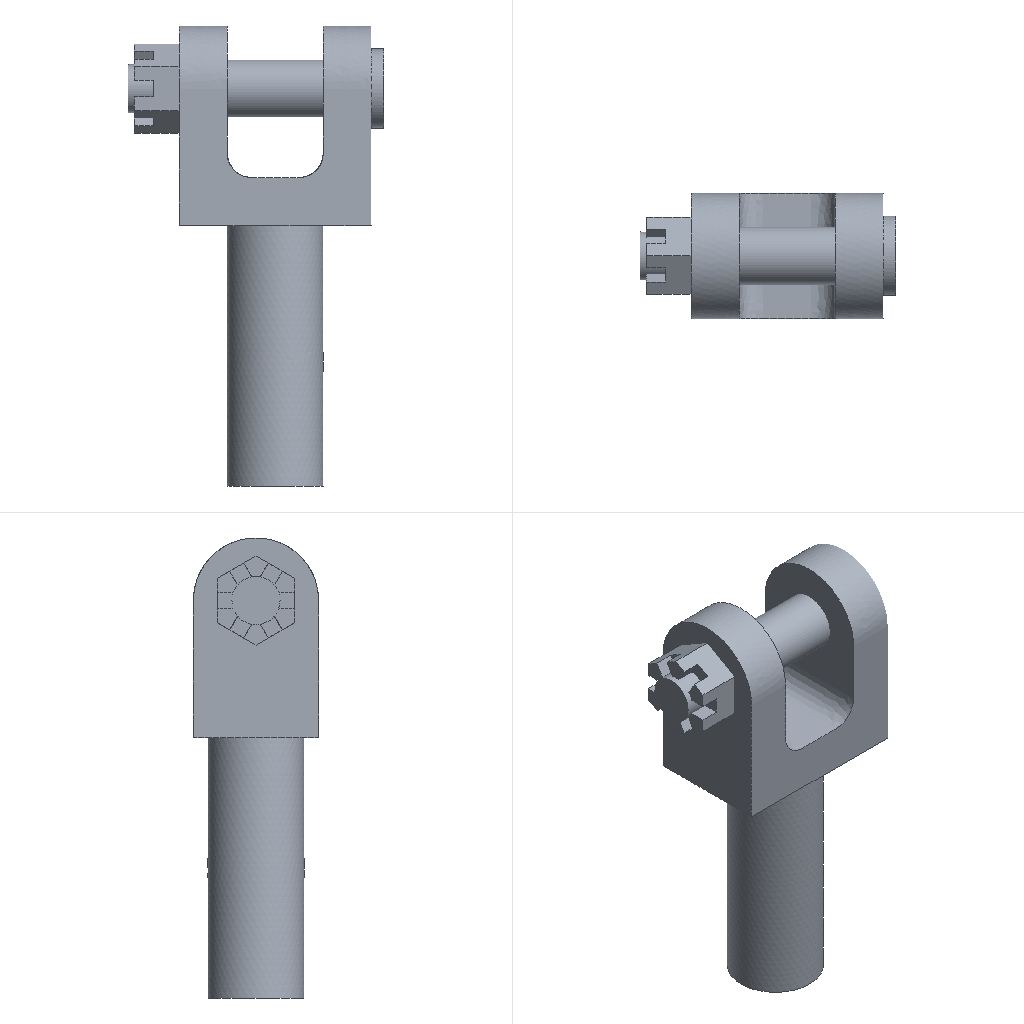Simulation study | ansys workbench
Set-up summary:
category,name,step,type,value,unit,region
solver,ansys_workbench
units,mm-N-s-tonne (MPa),,stated,"/units,MPA"
analysis,LS1,,static
load_step,LS1,LS1,static,nsubst=1; time=1
mesh,nodes,,,248082
mesh,elements,,,141187
element_type,SOLID187,,,108372
element_type,SOLID186,,,20185
element_type,TARGE170,,,5715
element_type,CONTA174,,,5715
element_type,SURF154,,,1200
material,Special steel,,E,200000,tonne s^-2 mm^-1
material,Special steel,,nu,0.3
material,Special steel,,density,7.85e-09,tonne mm^-3
load,Create Bearing Load,LS1,surface-effect pres face 5,65500,,SURF154 #12
bc,Fixed Supports,model,fixed,[dofs=ALL],,_FIXEDSU
bc,"Construct Weak Springs, Prototype 1",model,fixed,[dofs=ALL n=3],,node list
bc,"Construct Weak Springs, Prototype 2",model,fixed,[dofs=ALL n=3],,node list
bc,"Construct Weak Springs, Prototype 3",model,fixed,[dofs=ALL n=3],,node list
contact,Bonded - part.1 To part.2,,bonded (always),element=CONTA174
contact,Bonded - part.1 To part.3,,bonded (always),element=CONTA174
contact,Frictionless - part.3 To part.1,,standard (frictionless/frictional),element=CONTA174
contact,Bonded - part.3 To part.2,,bonded (always),element=CONTA174
named_set,_FIXEDSU,,node,6972
Ansys APDL input file, long lists of numbers shortened:
/batch
/config,noeldb,1     ! force off writing results to database
*get,_wallstrt,active,,time,wall
! ANSYS input file written by Workbench version 17.0 RELEASE
! File used for geometry attach:
/title,Hinge_pin_analysis--Static Structural (A5)
*DIM,_wb_ProjectScratch_dir,string,248
_wb_ProjectScratch_dir(1) = ''
*DIM,_wb_SolverFiles_dir,string,248
_wb_SolverFiles_dir(1) = ''
*DIM,_wb_userfiles_dir,string,248
_wb_userfiles_dir(1) = ''
/com,--- Data in consistent NMM units. See Solving Units in the help system for more information.
/units,MPA
/nopr
/wb,file,start              !  signify a WB generated input file
/prep7
! Turn off shape checking because checks already performed inside WB mesher.
! See help system for more information.
SHPP,OFF,,NOWARN
/nolist
etcon,set             ! allow ANSYS to choose best KEYOP's for 180x elements
/com,*********** Nodes for the whole assembly ***********
nblock,3
(1i9,3e20.9e3)
    88057   -2.930000000E+001   -2.527756814E+000    7.482179677E+001
! (248081 more lines like these left out)
-1
/wb,elem,start            !  set before creation of elements
/com,*********** Elements for Body 1 "part.1" ***********
et,1,187
eblock,19,solid,,98306
(19i9)
        1        1        1        1        0        0        0        0       10        0    30252   108013   108036   110488   110487   150708   150871   150712   150711
! (196611 more lines like these left out)
-1
/com,*********** Elements for Body 2 "part.2" ***********
et,2,187
eblock,19,solid,,10066
(19i9)
        2        2        2        2        0        0        0        0       10        0    20186    89367    90267    89959    90136    98772   102626    98769    98771
! (20131 more lines like these left out)
-1
/com,*********** Elements for Body 3 "part.3" ***********
et,3,186
keyo,3,2,1          ! set full integration on SOLID186
eblock,19,solid,,20185
(19i9)
        3        3        3        3        0        0        0        0       20        0   128558   270364   270368   270458   270457   270640   270644   270734   270733
! (40369 more lines like these left out)
-1
/wb,elem,end               !  done creating elements
/com,*********** Send User Defined Coordinate System(s) ***********
csys,0
toffst,273.15,  ! Temperature offset from absolute zero
/com,*********** Set Reference Temperature ***********
tref,22.
/wb,mat,start              !  starting to send materials
/com,*********** Send Materials ***********
MP,DENS,1,7.85e-09,	! tonne mm^-3
MP,EX,1,200000,	! tonne s^-2 mm^-1
MP,NUXY,1,0.3,
MP,DENS,2,7.85e-09,	! tonne mm^-3
MP,EX,2,200000,	! tonne s^-2 mm^-1
MP,NUXY,2,0.3,
MP,DENS,3,7.85e-09,	! tonne mm^-3
MP,EX,3,200000,	! tonne s^-2 mm^-1
MP,NUXY,3,0.3,
/wb,mat,end                !  done sending materials
!************************* Model Summary ********************
!part.1,	Special steel,	matid,	1
!part.2,	Special steel,	matid,	2
!part.3,	Special steel,	matid,	3
!************************* End Model Summary ********************
! get the diagonal of the bounding box. Needed later for other things
*get,_xmin,node,,mnloc,x
*get,_ymin,node,,mnloc,y
*get,_zmin,node,,mnloc,z
*get,_xmax,node,,mxloc,x
*get,_ymax,node,,mxloc,y
*get,_zmax,node,,mxloc,z
_ASMDIAG=(_xmax-_xmin)*(_xmax-_xmin)+(_ymax-_ymin)*(_ymax-_ymin)+(_zmax-_zmin)*(_zmax-_zmin)
_ASMDIAG=SQRT(_ASMDIAG)
/wb,contact,start          !  starting to send contact
/com,*********** Create Contact "Bonded - part.1 To part.2" ***********
/com,            Real Constant Set For Above Contact Is 5 & 4
*set,tid,5
*set,cid,4
r,tid
r,cid
et,tid,170
et,cid,174
eblock,10,,,201
(15i9)
   148743        5        5        5        0   109561   109894   109667   109667   161297   162289   109667   161294
! (200 more lines like these left out)
-1
eblock,10,,,201
(15i9)
   148944        4        4        4        0   109561   109894   109667   109667   161297   162289   109667   161294
! (200 more lines like these left out)
-1
eblock,10,,,318
(15i9)
   149145        4        5        4        0    88662    88692    88681    88681    94560    94724    88681    94558
! (317 more lines like these left out)
-1
eblock,10,,,318
(15i9)
   149463        5        4        5        0    88662    88692    88681    88681    94560    94724    88681    94558
! (317 more lines like these left out)
-1
keyo,cid,8,2               ! auto create asymmetric contact (from Program Controlled setting)
keyo,cid,10,2              ! adjust contact stiffness each NR iteration (from Program Controlled setting)
keyo,cid,12,5              ! bonded always
keyo,cid,2,0               ! augmented Lagrange (from Program Controlled setting)
keyo,cid,4,0               ! on Gauss point (from Program Controlled setting)
keyo,cid,9,1               ! ignore initial gaps/penetration
keyo,cid,7,0               ! No Prediction
rmod,tid,3,1.	! FKN
rmod,tid,5,0.	! ICONT
rmod,tid,6,0.	! PINB
rmod,tid,10,0.	! CNOF
rmod,tid,12,0.	! FKT
rmod,tid,36,455	! WB DSID
rmod,cid,3,1.	! FKN
rmod,cid,5,0.	! ICONT
rmod,cid,6,0.	! PINB
rmod,cid,10,0.	! CNOF
rmod,cid,12,0.	! FKT
rmod,cid,36,455	! WB DSID
/com,*********** Create Contact "Bonded - part.1 To part.3" ***********
/com,            Real Constant Set For Above Contact Is 7 & 6
*set,tid,7
*set,cid,6
r,tid
r,cid
et,tid,170
et,cid,174
eblock,10,,,870
(15i9)
   149781        7        7        7        0   108776   109073   108950   108950   156013   157507   108950   156011
! (869 more lines like these left out)
-1
eblock,10,,,870
(15i9)
   150651        6        6        6        0   108776   109073   108950   108950   156013   157507   108950   156011
! (869 more lines like these left out)
-1
eblock,10,,,120
(15i9)
   151521        6        7        6        0   248190   248189   248434   248441   271549   272020   272040   270858
! (119 more lines like these left out)
-1
eblock,10,,,120
(15i9)
   151641        7        6        7        0   248190   248189   248434   248441   271549   272020   272040   270858
! (119 more lines like these left out)
-1
keyo,cid,8,2               ! auto create asymmetric contact (from Program Controlled setting)
keyo,cid,10,2              ! adjust contact stiffness each NR iteration (from Program Controlled setting)
keyo,cid,12,5              ! bonded always
keyo,cid,2,0               ! augmented Lagrange (from Program Controlled setting)
keyo,cid,4,0               ! on Gauss point (from Program Controlled setting)
keyo,cid,9,1               ! ignore initial gaps/penetration
keyo,cid,7,0               ! No Prediction
rmod,tid,3,1.	! FKN
rmod,tid,5,0.	! ICONT
rmod,tid,6,0.	! PINB
rmod,tid,10,0.	! CNOF
rmod,tid,12,0.	! FKT
rmod,tid,36,461	! WB DSID
rmod,cid,3,1.	! FKN
rmod,cid,5,0.	! ICONT
rmod,cid,6,0.	! PINB
rmod,cid,10,0.	! CNOF
rmod,cid,12,0.	! FKT
rmod,cid,36,461	! WB DSID
/com,*********** Create Contact "Frictionless - part.3 To part.1" ***********
/com,            Real Constant Set For Above Contact Is 9 & 8
*set,tid,9
*set,cid,8
r,tid
r,cid
et,tid,170
et,cid,174
eblock,10,,,2400
(15i9)
   151761        9        9        9        0   255215   255551   255550   255214   291870   291869   291868   270949
! (2399 more lines like these left out)
-1
eblock,10,,,2400
(15i9)
   154161        8        8        8        0   255215   255551   255550   255214   291870   291869   291868   270949
! (2399 more lines like these left out)
-1
eblock,10,,,728
(15i9)
   156561        8        9        8        0   104315   104417   104210   104210   124699   123907   104210   123906
! (727 more lines like these left out)
-1
eblock,10,,,728
(15i9)
   157289        9        8        9        0   104315   104417   104210   104210   124699   123907   104210   123906
! (727 more lines like these left out)
-1
keyo,cid,8,2               ! auto create asymmetric contact (from Program Controlled setting)
keyo,cid,10,2              ! adjust contact stiffness each NR iteration (from Program Controlled setting)
keyo,cid,12,0              ! standard contact
keyo,cid,2,0               ! augmented Lagrange (from Program Controlled setting)
keyo,cid,4,0               ! on Gauss point (from Program Controlled setting)
keyo,cid,9,0               ! use real geometry with stepped effects
keyo,cid,7,0               ! No Prediction
rmod,tid,3,1.	! FKN
rmod,tid,5,0.	! ICONT
rmod,tid,6,0.	! PINB
rmod,tid,10,0.	! CNOF
rmod,tid,12,0.	! FKT
rmod,tid,36,506	! WB DSID
rmod,cid,3,1.	! FKN
rmod,cid,5,0.	! ICONT
rmod,cid,6,0.	! PINB
rmod,cid,10,0.	! CNOF
rmod,cid,12,0.	! FKT
rmod,cid,36,506	! WB DSID
/com,*********** Create Contact "Bonded - part.3 To part.2" ***********
/com,            Real Constant Set For Above Contact Is 11 & 10
*set,tid,11
*set,cid,10
r,tid
r,cid
et,tid,170
et,cid,174
eblock,10,,,600
(15i9)
   158017       11       11       11        0   248812   248814   248813   248811   272958   272956   272955   271382
! (599 more lines like these left out)
-1
eblock,10,,,600
(15i9)
   158617       10       10       10        0   248812   248814   248813   248811   272958   272956   272955   271382
! (599 more lines like these left out)
-1
eblock,10,,,478
(15i9)
   159217       10       11       10        0    88211    88212    88467    88467    91383    91393    88467    91386
! (477 more lines like these left out)
-1
eblock,10,,,478
(15i9)
   159695       11       10       11        0    88211    88212    88467    88467    91383    91393    88467    91386
! (477 more lines like these left out)
-1
keyo,cid,8,2               ! auto create asymmetric contact (from Program Controlled setting)
keyo,cid,10,2              ! adjust contact stiffness each NR iteration (from Program Controlled setting)
keyo,cid,12,5              ! bonded always
keyo,cid,2,0               ! augmented Lagrange (from Program Controlled setting)
keyo,cid,4,0               ! on Gauss point (from Program Controlled setting)
keyo,cid,9,1               ! ignore initial gaps/penetration
keyo,cid,7,0               ! No Prediction
rmod,tid,3,1.	! FKN
rmod,tid,5,0.	! ICONT
rmod,tid,6,0.	! PINB
rmod,tid,10,0.	! CNOF
rmod,tid,12,0.	! FKT
rmod,tid,36,510	! WB DSID
rmod,cid,3,1.	! FKN
rmod,cid,5,0.	! ICONT
rmod,cid,6,0.	! PINB
rmod,cid,10,0.	! CNOF
rmod,cid,12,0.	! FKT
rmod,cid,36,510	! WB DSID
nsel,all
esel,all
/wb,contact,end            !  done creating contacts
/golist
/wb,load,start             !  starting to send loads
/com,*********** Fixed Supports ***********
CMBLOCK,_FIXEDSU,NODE,     6972
(8i10)
    104728    104729    104730    104731    104732    104733    104734    104735
! (871 more lines like these left out)
cmsel,s,_FIXEDSU
d,all,all
nsel,all
nsel,all
/com,*********** Create Bearing Load ***********
et,12,154
eblock,10,,,1200
(15i9)
   160173       12       12       12        0   255192   255528   255527   255191   291818   291817   270989   271247
! (1199 more lines like these left out)
-1
esel,s,type,,12
keyop,12,7,1                ! Use original area so load is constant in large deformation
esel,all
et,13,14             ! spring element type
/com,*********** Construct Weak Springs, Prototype 1 ***********
*set,_delta,5.342
type,13
mat,14
real,14
r,14,1.45131937772807e-004
nsel,all
*get,_nspr,ndmx
_nspr=_nspr+1
esel,s,mat,,1
nsle,s,active
*get,_minx,node,0,mnloc,x
*get,_miny,node,0,mnloc,y
*get,_minz,node,0,mnloc,z
*get,_maxx,node,0,mxloc,x
*get,_maxy,node,0,mxloc,y
*get,_maxz,node,0,mxloc,z
*dim,_ntets,arra,8
_ntets(1) = NODE(_minx,_miny,_minz)
_ntets(2) = NODE(_minx,_miny,_maxz)
_ntets(3) = NODE(_minx,_maxy,_minz)
_ntets(4) = NODE(_minx,_maxy,_maxz)
_ntets(5) = NODE(_maxx,_miny,_minz)
_ntets(6) = NODE(_maxx,_miny,_maxz)
_ntets(7) = NODE(_maxx,_maxy,_minz)
_ntets(8) = NODE(_maxx,_maxy,_maxz)
*do,_i,1,8
  n,_nspr,nx(_ntets(_i))+_delta,ny(_ntets(_i)),nz(_ntets(_i))
  e,_ntets(_i),_nspr
  d,_nspr,all
  _nspr=_nspr+1
  n,_nspr,nx(_ntets(_i)),ny(_ntets(_i))+_delta,nz(_ntets(_i))
  e,_ntets(_i),_nspr
  d,_nspr,all
  _nspr=_nspr+1
  n,_nspr,nx(_ntets(_i)),ny(_ntets(_i)),nz(_ntets(_i))+_delta
  e,_ntets(_i),_nspr
  d,_nspr,all
  _nspr=_nspr+1
*enddo
*set,_ntets
nsel,all
esel,all
/com,*********** Construct Weak Springs, Prototype 2 ***********
*set,_delta,1.308
type,13
mat,15
real,15
r,15,9.49946830519664e-005
nsel,all
*get,_nspr,ndmx
_nspr=_nspr+1
esel,s,mat,,2
nsle,s,active
*get,_minx,node,0,mnloc,x
*get,_miny,node,0,mnloc,y
*get,_minz,node,0,mnloc,z
*get,_maxx,node,0,mxloc,x
*get,_maxy,node,0,mxloc,y
*get,_maxz,node,0,mxloc,z
*dim,_ntets,arra,8
_ntets(1) = NODE(_minx,_miny,_minz)
_ntets(2) = NODE(_minx,_miny,_maxz)
_ntets(3) = NODE(_minx,_maxy,_minz)
_ntets(4) = NODE(_minx,_maxy,_maxz)
_ntets(5) = NODE(_maxx,_miny,_minz)
_ntets(6) = NODE(_maxx,_miny,_maxz)
_ntets(7) = NODE(_maxx,_maxy,_minz)
_ntets(8) = NODE(_maxx,_maxy,_maxz)
*do,_i,1,8
  n,_nspr,nx(_ntets(_i))+_delta,ny(_ntets(_i)),nz(_ntets(_i))
  e,_ntets(_i),_nspr
  d,_nspr,all
  _nspr=_nspr+1
  n,_nspr,nx(_ntets(_i)),ny(_ntets(_i))+_delta,nz(_ntets(_i))
  e,_ntets(_i),_nspr
  d,_nspr,all
  _nspr=_nspr+1
  n,_nspr,nx(_ntets(_i)),ny(_ntets(_i)),nz(_ntets(_i))+_delta
  e,_ntets(_i),_nspr
  d,_nspr,all
  _nspr=_nspr+1
*enddo
*set,_ntets
nsel,all
esel,all
/com,*********** Construct Weak Springs, Prototype 3 ***********
*set,_delta,2.895
type,13
mat,16
real,16
r,16,1.31071703429123e-004
nsel,all
*get,_nspr,ndmx
_nspr=_nspr+1
esel,s,mat,,3
nsle,s,active
*get,_minx,node,0,mnloc,x
*get,_miny,node,0,mnloc,y
*get,_minz,node,0,mnloc,z
*get,_maxx,node,0,mxloc,x
*get,_maxy,node,0,mxloc,y
*get,_maxz,node,0,mxloc,z
*dim,_ntets,arra,8
_ntets(1) = NODE(_minx,_miny,_minz)
_ntets(2) = NODE(_minx,_miny,_maxz)
_ntets(3) = NODE(_minx,_maxy,_minz)
_ntets(4) = NODE(_minx,_maxy,_maxz)
_ntets(5) = NODE(_maxx,_miny,_minz)
_ntets(6) = NODE(_maxx,_miny,_maxz)
_ntets(7) = NODE(_maxx,_maxy,_minz)
_ntets(8) = NODE(_maxx,_maxy,_maxz)
*do,_i,1,8
  n,_nspr,nx(_ntets(_i))+_delta,ny(_ntets(_i)),nz(_ntets(_i))
  e,_ntets(_i),_nspr
  d,_nspr,all
  _nspr=_nspr+1
  n,_nspr,nx(_ntets(_i)),ny(_ntets(_i))+_delta,nz(_ntets(_i))
  e,_ntets(_i),_nspr
  d,_nspr,all
  _nspr=_nspr+1
  n,_nspr,nx(_ntets(_i)),ny(_ntets(_i)),nz(_ntets(_i))+_delta
  e,_ntets(_i),_nspr
  d,_nspr,all
  _nspr=_nspr+1
*enddo
*set,_ntets
nsel,all
esel,all
/gst,on,on
fini
*get,_numnode,node,0,count
*get,_numelem,elem,0,count
*get, _MAXELEMNUM, elem, 0, NUM, MAX
*get, _MAXNODENUM, node, 0, NUM, MAX
*get, _MAXELEMTYPE, etyp, 0, NUM, MAX
*get, _MAXREALCONST, real, 0, NUM, MAX
/go
/wb,load,end               !  done creating loads
/com,--- Number of total nodes = %_numnode%
/com,--- Number of contact elements = 12630
/com,--- Number of spring elements = 72
/com,--- Number of bearing elements = 0
/com,--- Number of solid elements = 128557
/com,--- Number of total elements = %_numelem%
*get,_wallbsol,active,,time,wall
/com,****************************************************************************
/com,*************************    SOLUTION       ********************************
/com,****************************************************************************
/solu
antype,0                   ! static analysis
eqsl,pcg,1e-8,,,,,,1
cntr,print,1               ! print out contact info and also make no initial contact an error
dmpopt,emat,no             ! Don't combine emat file for DANSYS
dmpopt,esav,no             ! Don't combine esav file for DANSYS
nldiag,cont,iter           ! print out contact info each equilibrium iteration
resc,define,last,last,,dele	   ! Program Controlled
/com,****************************************************
/com,******************* SOLVE FOR LS 1 ****************
esel,s,type,,12
sfe,all,5,pres,0,0.0,1.,0.,0.
local,11,0,0,0,0,90.,0.,-90.
csys,0
*set,_v1,0.
*set,_v2,0.
*set,_v3,1.
*get,_necurr,elem,,count
_ecurr=0
_total=0
*do,_i,1,_necurr
  _ecurr = ELNEXT(_ecurr)
  _normx = NORMNX(NELEM(_ecurr,1),NELEM(_ecurr,2),NELEM(_ecurr,3))
! (7 more lines like these left out)
  *if,_dot,gt,-0.00001,then
    esel,u,elem,,_ecurr
  *else
    csys,11
    *get,_indd,elem,_ecurr,aproj,x
    csys,0
    _total=_total+_indd
  *endif
*enddo
*get,_necurr,elem,,count
*if,_necurr,eq,0,then
  *msg,error
  NO ELEMENTS ARE SELECTED TO APPLY BEARING LOAD TO. &
  IT IS LIKELY THAT THE BEARING LOAD IS IN THE WRONG DIRECTION
*endif
*set,_mag,65500.
_mag=_mag/_total
sfe,all,5,pres,0,_mag,0.,0.,65500.
nsel,all
esel,all
/nopr
/gopr
autots,on                  ! Workbench Program Controlled automatic time stepping
nsub,1,10,1                ! due to presence of general nonlinear
time,1.
outres,erase
outres,all,none
outres,nsol,all
outres,rsol,all
outres,strs,all
outres,epel,all
outres,eppl,all
stabilize,off                   ! Stabilization turned OFF by user
! *********** WB SOLVE COMMAND ***********
! check interactive state
*get,ANSINTER_,active,,int
*if,ANSINTER_,ne,0,then
/eof
*endif
solve
/com *************** Write FE CONNECTORS *********
CEWRITE,file,ce,,INTE
/com,****************************************************
/com,*************** FINISHED SOLVE FOR LS 1 *************
*set,_DS_PROGRESS          ! turn off progress updates to avoid virus scanning bug
*get,_wallasol,active,,time,wall
/nopr
*get,_numnode,node,0,count
*get,_numelem,elem,0,count
*get, _MAXELEMNUM, elem, 0, NUM, MAX
*get, _MAXNODENUM, node, 0, NUM, MAX,,,INTERNAL
*get, _MAXELEMTYPE, etyp, 0, NUM, MAX
*get, _MAXREALCONST, real, 0, NUM, MAX
/gopr
*get,_PCGITER,active,,solu,cgiter
/post1
xmlo,ENCODING,ISO-8859-1
xmlo,parm
/xml,parm,xml
fini
/gopr
*get,_walldone,active,,time,wall
_preptime=(_wallbsol-_wallstrt)*3600
_solvtime=(_wallasol-_wallbsol)*3600
_posttime=(_walldone-_wallasol)*3600
_totaltim=(_walldone-_wallstrt)*3600
/wb,file,end               ! done with WB generated input
Results summary:
result,analyses[0].index,,,1
result,analyses[0].system,,,SYS-1
result,analyses[0].deck,,,deck.dat
result,analyses[0].solve_status,,,completed
result,analyses[0].analysis_type,,,static
result,analyses[0].physics,,,mechanical
result,analyses[0].unit_system,,,"NMM: mm, ton, N, s, mV, mA, degC"
result,analyses[0].n_sets,,,1
result,analyses[0].load_steps[0].set,set=1,,1
result,analyses[0].load_steps[0].time_or_freq,set=1,,1
result,analyses[0].load_steps[0].max_displacement_magnitude,set=1,,0.1504
result,analyses[0].load_steps[0].max_von_mises_nodal,set=1,,1563.52
result,analyses[0].load_steps[0].reaction_force_sum_xyz[1],set=1,,-4.32249e-09
result,analyses[0].load_steps[0].reaction_force_sum_xyz[2],set=1,,-3.94528e-09
result,analyses[0].load_steps[0].reaction_force_sum_xyz[3],set=1,,-65500
result,geometry_export[0][0],,,.step
result,geometry_export[0][1],,,ok
result,geometry_export[0][2],,,3